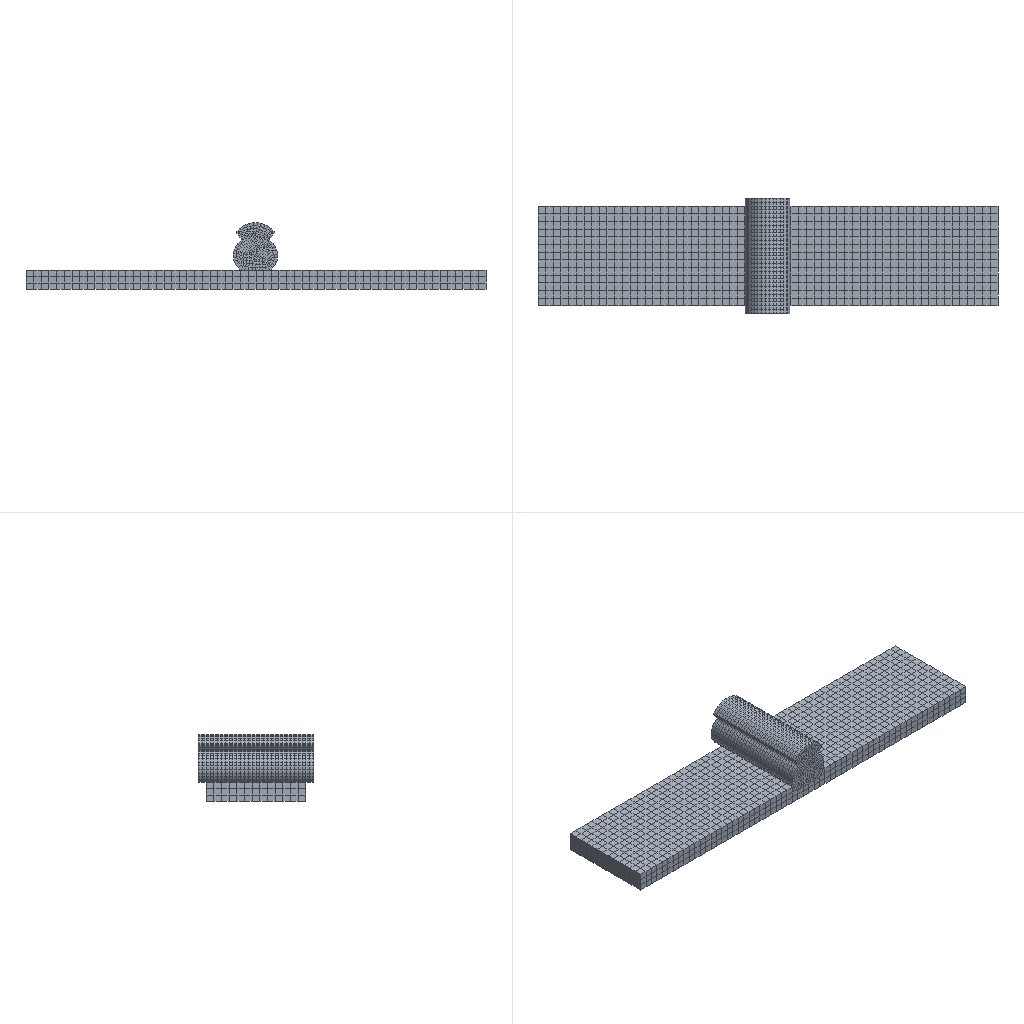Simulation study | abaqus
Set-up summary:
category,name,step,type,value,unit,region
solver,abaqus
solver,version,,,Abaqus/Standard 2020
units,not stated in the deck,,not stated
analysis,deck,,coupled thermal-electrical,coupled thermal-electrical
load_step,Step-1,Step-1,coupled thermal-electrical
load_step,requested,,,1
mesh,nodes,,,13119
mesh,elements,,,10950
element_type,DC3D8E,,solid,10950
load,load commands in deck,,count,3
bc,support commands in deck,,count,4
material,TAN,,in results
material,XIAN,,in results
check,setup vs results,,match,"per instance, exact: element labels, types and connectivity; labels of the nodes the elements use; coordinates not compared"
Abaqus input file, long lists of numbers shortened:
*Heading
** Job name: Job-another Model name: Model-1-another
** Generated by: Abaqus/CAE 2020
*Preprint, echo=NO, model=NO, history=NO, contact=NO
**
** PARTS
**
*Part, name=P222
*Node
      1,         120.,         -23.,           5.
      2,         120.,         -23.,   3.333
** (3414 more lines like these left out)
*Element, type=DC3D8E
   1,   57,   58,   62,   61,    1,    2,    6,    5
   2,   58,   59,   63,   62,    2,    3,    7,    6
** (2338 more lines like these left out)
*Nset, nset=Set-2, generate
    1,  3416,     1
*Elset, elset=Set-2, generate
    1,  2340,     1
** Section: tan
*Solid Section, elset=Set-2, material=tan
,
*End Part
**
*Part, name=dao
*Node
      1,  -3.661,   2.151,           0.
      2,  -4.726,   3.409,           0.
** (9701 more lines like these left out)
*Element, type=DC3D8E
   1,   60,    4,    3,   56,  373,  317,  316,  369
   2,    3,    2,  273,   56,  316,  315,  586,  369
** (8608 more lines like these left out)
*Nset, nset=Set-3, generate
    1,  9703,     1
*Elset, elset=Set-3, generate
    1,  8610,     1
** Section: xian
*Solid Section, elset=Set-3, material=xian
,
*End Part
**
**
** ASSEMBLY
**
*Assembly, name=Assembly
**
*Instance, name=P222-1, part=P222
*End Instance
**
*Instance, name=dao-1, part=dao
   59.767,           5.,    11.079
   59.767,           5.,    11.079, 60.767,           5.,    11.079, 90.
*End Instance
**
*Nset, nset=Set-1, instance=P222-1, generate
    1,  3416,     1
*Nset, nset=Set-1, instance=dao-1
    1,   30,   31,  314,  343,  344,  627,  656,  657,  940,  969,  970, 1253, 1282, 1283, 1566
 1595, 1596, 1879, 1908, 1909, 2192, 2221, 2222, 2505, 2534, 2535, 2818, 2847, 2848, 3131, 3160
** (4 more lines like these left out)
*Elset, elset=Set-1, instance=P222-1, generate
    1,  2340,     1
*Elset, elset=Set-1, instance=dao-1
   12,   47,  186,  299,  334,  473,  586,  621,  760,  873,  908, 1047, 1160, 1195, 1334, 1447
 1482, 1621, 1734, 1769, 1908, 2021, 2056, 2195, 2308, 2343, 2482, 2595, 2630, 2769, 2882, 2917
** (4 more lines like these left out)
*Nset, nset=Set-3, instance=P222-1, generate
    1,  3416,     1
*Elset, elset=Set-3, instance=P222-1, generate
    1,  2340,     1
*Nset, nset=Set-5, instance=dao-1
    1,    2,   13,   14,   32,   33,   38,  314,  315,  326,  327,  345,  346,  351,  627,  628
  639,  640,  658,  659,  664,  940,  941,  952,  953,  971,  972,  977, 1253, 1254, 1265, 1266
** (12 more lines like these left out)
*Elset, elset=Set-5, instance=dao-1
    3,   13,  182,  183,  277,  290,  300,  469,  470,  564,  577,  587,  756,  757,  851,  864
  874, 1043, 1044, 1138, 1151, 1161, 1330, 1331, 1425, 1438, 1448, 1617, 1618, 1712, 1725, 1735
** (8 more lines like these left out)
*Nset, nset=Set-6, instance=dao-1, generate
   1,  313,    1
*Elset, elset=Set-6, instance=dao-1, generate
   1,  287,    1
*Elset, elset=_Surf-2_S3, internal, instance=P222-1
    1,    2,    3,   40,   41,   42,   79,   80,   81,  118,  119,  120,  157,  158,  159,  196
  197,  198,  235,  236,  237,  274,  275,  276,  313,  314,  315,  352,  353,  354,  391,  392
** (10 more lines like these left out)
*Elset, elset=_Surf-2_S5, internal, instance=P222-1
   37,   38,   39,   76,   77,   78,  115,  116,  117,  154,  155,  156,  193,  194,  195,  232
  233,  234,  271,  272,  273,  310,  311,  312,  349,  350,  351,  388,  389,  390,  427,  428
** (10 more lines like these left out)
*Elset, elset=_Surf-2_S5, internal, instance=dao-1
   12,   47,  299,  334,  586,  621,  873,  908, 1160, 1195, 1447, 1482, 1734, 1769, 2021, 2056
 2308, 2343, 2595, 2630, 2882, 2917, 3169, 3204, 3456, 3491, 3743, 3778, 4030, 4065, 4317, 4352
** (2 more lines like these left out)
*Elset, elset=_Surf-2_S1, internal, instance=P222-1, generate
 2302,  2340,     1
*Elset, elset=_Surf-2_S4, internal, instance=P222-1, generate
    3,  2340,     3
*Elset, elset=_Surf-2_S2, internal, instance=P222-1, generate
  1,  39,   1
*Elset, elset=_Surf-2_S6, internal, instance=P222-1, generate
    1,  2338,     3
*Surface, type=ELEMENT, name=Surf-2
_Surf-2_S3, S3
_Surf-2_S5, S5
_Surf-2_S4, S4
_Surf-2_S2, S2
_Surf-2_S6, S6
_Surf-2_S1, S1
*Elset, elset=_Surf-3_S3, internal, instance=P222-1
    1,    2,    3,   40,   41,   42,   79,   80,   81,  118,  119,  120,  157,  158,  159,  196
  197,  198,  235,  236,  237,  274,  275,  276,  313,  314,  315,  352,  353,  354,  391,  392
** (10 more lines like these left out)
*Elset, elset=_Surf-3_S5, internal, instance=P222-1
   37,   38,   39,   76,   77,   78,  115,  116,  117,  154,  155,  156,  193,  194,  195,  232
  233,  234,  271,  272,  273,  310,  311,  312,  349,  350,  351,  388,  389,  390,  427,  428
** (10 more lines like these left out)
*Elset, elset=_Surf-3_S5, internal, instance=dao-1
   12,   47,  299,  334,  586,  621,  873,  908, 1160, 1195, 1447, 1482, 1734, 1769, 2021, 2056
 2308, 2343, 2595, 2630, 2882, 2917, 3169, 3204, 3456, 3491, 3743, 3778, 4030, 4065, 4317, 4352
** (2 more lines like these left out)
*Elset, elset=_Surf-3_S1, internal, instance=P222-1, generate
 2302,  2340,     1
*Elset, elset=_Surf-3_S4, internal, instance=P222-1, generate
    3,  2340,     3
*Elset, elset=_Surf-3_S2, internal, instance=P222-1, generate
  1,  39,   1
*Elset, elset=_Surf-3_S6, internal, instance=P222-1, generate
    1,  2338,     3
*Surface, type=ELEMENT, name=Surf-3
_Surf-3_S3, S3
_Surf-3_S5, S5
_Surf-3_S4, S4
_Surf-3_S2, S2
_Surf-3_S6, S6
_Surf-3_S1, S1
*Elset, elset=_Surf-6_S2, internal, instance=dao-1, generate
 8324,  8610,     1
*Surface, type=ELEMENT, name=Surf-6
_Surf-6_S2, S2
*Elset, elset=_m_Surf-7_S3, internal, instance=dao-1
   36,  171,  234,  235,  239,  323,  458,  521,  522,  526,  610,  745,  808,  809,  813,  897
 1032, 1095, 1096, 1100, 1184, 1319, 1382, 1383, 1387, 1471, 1606, 1669, 1670, 1674, 1758, 1893
** (8 more lines like these left out)
*Elset, elset=_m_Surf-7_S5, internal, instance=dao-1
   94,  244,  245,  381,  531,  532,  668,  818,  819,  955, 1105, 1106, 1242, 1392, 1393, 1529
 1679, 1680, 1816, 1966, 1967, 2103, 2253, 2254, 2390, 2540, 2541, 2677, 2827, 2828, 2964, 3114
** (4 more lines like these left out)
*Surface, type=ELEMENT, name=m_Surf-7
_m_Surf-7_S3, S3
_m_Surf-7_S5, S5
*Elset, elset=_s_Surf-4_S6, internal, instance=P222-1, generate
    1,  2338,     3
*Surface, type=ELEMENT, name=s_Surf-4
_s_Surf-4_S6, S6
** Constraint: Constraint-1
*Tie, name=Constraint-1, adjust=yes
s_Surf-4, m_Surf-7
*End Assembly
**
** MATERIALS
**
*Material, name=tan
*Conductivity
3.,
*Density
 1.67e-09,
*Elastic
36500., 0.425
*Electrical Conductivity
 0.0005,
*Expansion
 3.5e-06,
*Specific Heat
 7.69e+08,
*Material, name=xian
*Conductivity
390.,
*Density
 8.9e-09,
*Elastic
110000., 0.32
*Electrical Conductivity
 0.002,
*Expansion
 1.66e-06,
*Plastic
250.,0.
*Specific Heat
 3.84e+08,
**
** PHYSICAL CONSTANTS
**
*Physical Constants, absolute zero=-273., stefan boltzmann=5.67e-08
**
** BOUNDARY CONDITIONS
**
** Name: BC-1 Type: 对称/反对称/完全固定
*Boundary
Set-5, ENCASTRE
**
** PREDEFINED FIELDS
**
** Name: Predefined Field-1   Type: Temperature
*Initial Conditions, type=TEMPERATURE
Set-1, 25.
** ----------------------------------------------------------------
**
** STEP: Step-1
**
*Step, name=Step-1, nlgeom=NO, inc=10000
*Coupled Thermal-electrical, steady state, deltmx=100000., mxdem=1.
1., 6000., 0.06, 6000.,
**
** BOUNDARY CONDITIONS
**
** Name: BC-2 Type: 电势
*Boundary
Set-6, 9, 9
**
** LOADS
**
** Name: Load-1   Type: Surface current
*Dsecurrent
Surf-6,CS,1.
**
** INTERACTIONS
**
** Interaction: Int-1
*Sradiate
Surf-2, R, 25., 0.1
** Interaction: Int-2
*Sfilm
Surf-3, F, 25., 0.2
**
** OUTPUT REQUESTS
**
*Restart, write, frequency=0
**
** FIELD OUTPUT: F-Output-1
**
*Output, field
*Node Output
CECHG, CECUR, EPOT, NT, RFL
*Element Output, directions=YES
ECD, EPG, HFL, TEMP
*Contact Output
ECD,
**
** HISTORY OUTPUT: H-Output-1
**
*Output, history, variable=PRESELECT
*End Step
Results summary:
result,step,,partial,increments=0 time=0.0/6000.0
result,analysis,,,"coupled thermal-electrical, steady state"
result,last_loadstep,,,1
result,primary field,,,"EPOT, NT11"